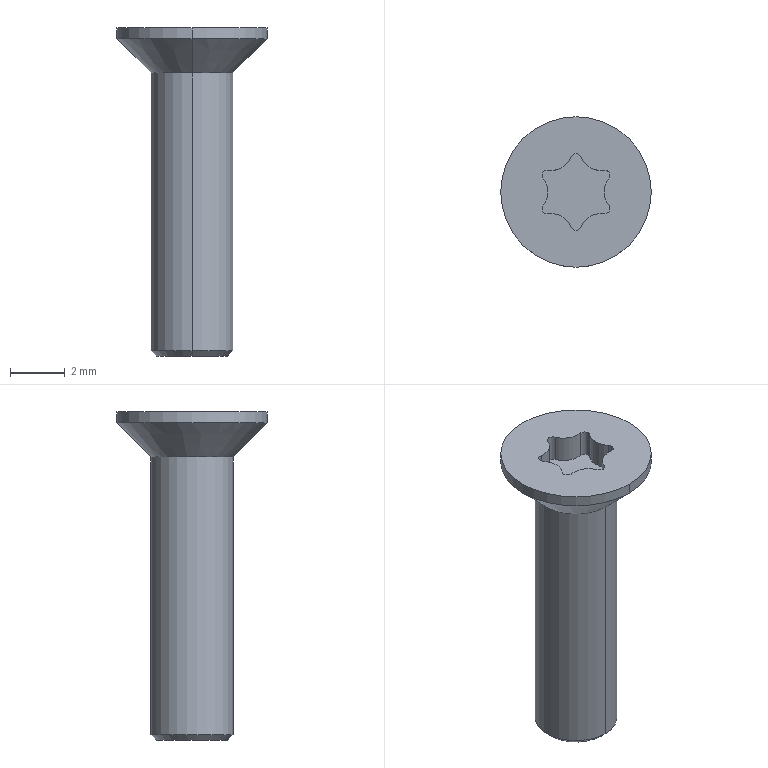Part | STEP file | ASND-0110-0219110003 | 1 solid | 26 faces | box 5.5 x 5.5 x 12 mm | volume 96.355 mm3 | cylinder 19 | cone 4 | plane 3 | commonest cylinder face diameters 0.4 x8 1.495 x7 3 x2 5.5 x2